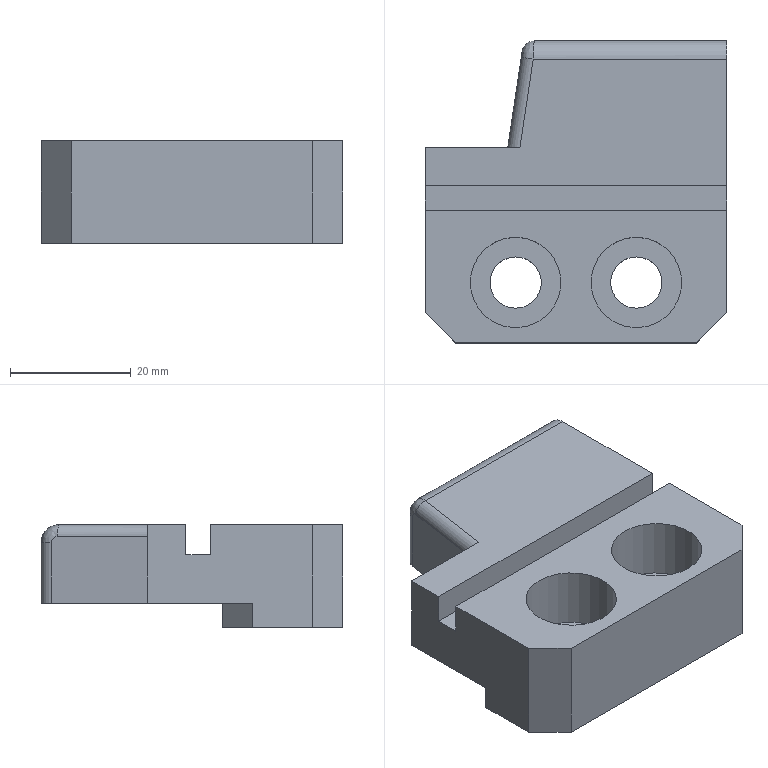Part | STEP file | gslz 2016.10.28-13_id334_x_t | 1 solid | 28 faces | box 50 x 50 x 17 mm | volume 27113 mm3 | plane 20 | cylinder 7 | spline 1 | commonest cylinder face diameters 4 x2 8.5 x2 15 x2 6 x1